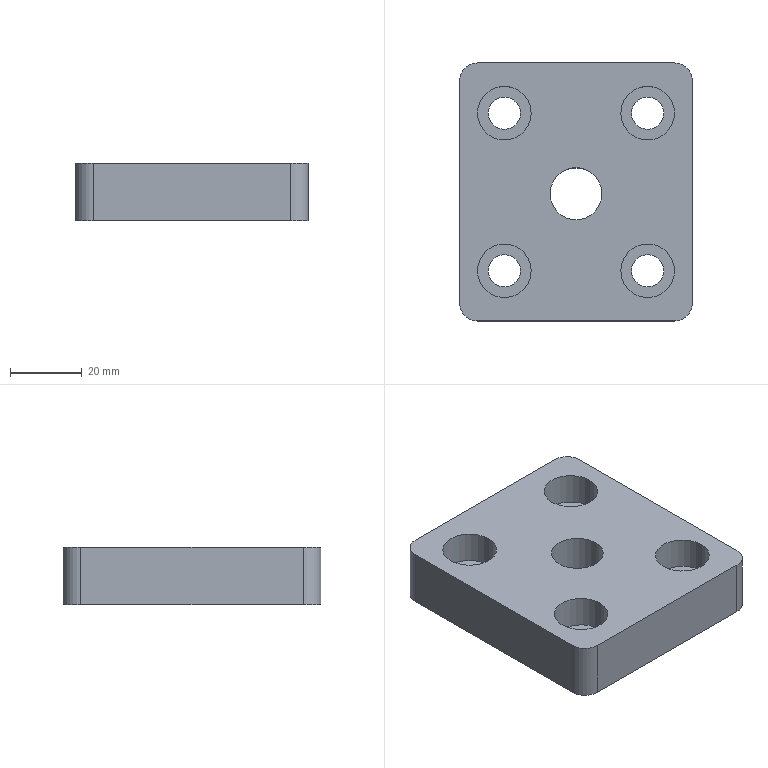Part | NX | features BREP 1 | 1 solid | 32 faces | box 65 x 72 x 16 mm | volume 63752 mm3 | cylinder 22 | plane 10 | commonest cylinder face diameters 9 x8 15 x8 10 x4 14.5 x2
STEP:
#1=CARTESIAN_POINT('',(7.25,-0.5,0.));
#2=VERTEX_POINT('',#1);
#3=CARTESIAN_POINT('',(-7.25,-0.5,0.));
#4=VERTEX_POINT('',#3);
#5=CARTESIAN_POINT('',(-0.000000218,-0.5,0.));
#6=DIRECTION('',(0.,0.,-1.));
#7=DIRECTION('',(-1.,0.,0.));
#8=AXIS2_PLACEMENT_3D('',#5,#6,#7);
#9=CIRCLE('',#8,7.25);
#10=EDGE_CURVE('',#2,#4,#9,.T.);
#11=ORIENTED_EDGE('',*,*,#10,.T.);
#12=CARTESIAN_POINT('',(-7.25,-0.5,16.));
#13=VERTEX_POINT('',#12);
#14=CARTESIAN_POINT('',(-7.25,-0.5,16.));
#15=DIRECTION('',(0.,0.,1.));
#16=VECTOR('',#15,1000.);
#17=LINE('',#14,#16);
#18=EDGE_CURVE('',#13,#4,#17,.F.);
#19=ORIENTED_EDGE('',*,*,#18,.F.);
#20=CARTESIAN_POINT('',(7.25,-0.5,16.));
#21=VERTEX_POINT('',#20);
#22=CARTESIAN_POINT('',(-0.000000218,-0.5,16.));
#23=DIRECTION('',(0.,0.,1.));
#24=DIRECTION('',(1.,0.,0.));
#25=AXIS2_PLACEMENT_3D('',#22,#23,#24);
#26=CIRCLE('',#25,7.25);
#27=EDGE_CURVE('',#13,#21,#26,.T.);
#28=ORIENTED_EDGE('',*,*,#27,.T.);
#29=CARTESIAN_POINT('',(7.25,-0.5,16.));
#30=DIRECTION('',(0.,0.,1.));
#31=VECTOR('',#30,1000.);
#32=LINE('',#29,#31);
#33=EDGE_CURVE('',#21,#2,#32,.F.);
#34=ORIENTED_EDGE('',*,*,#33,.T.);
#35=EDGE_LOOP('',(#11,#19,#28,#34));
#36=FACE_BOUND('',#35,.T.);
#37=CARTESIAN_POINT('',(-0.000000218,-0.5,16.));
#38=DIRECTION('',(0.,0.,1.));
#39=DIRECTION('',(1.,0.,0.));
#40=AXIS2_PLACEMENT_3D('',#37,#38,#39);
#41=CYLINDRICAL_SURFACE('',#40,7.25);
#42=ADVANCED_FACE('',(#36),#41,.F.);
#43=CARTESIAN_POINT('',(-27.5,22.,7.));
#44=VERTEX_POINT('',#43);
#45=CARTESIAN_POINT('',(-12.5,22.,7.));
#46=VERTEX_POINT('',#45);
#47=CARTESIAN_POINT('',(-20.,22.,7.));
#48=DIRECTION('',(0.,0.,1.));
#49=DIRECTION('',(1.,0.,0.));
#50=AXIS2_PLACEMENT_3D('',#47,#48,#49);
#51=CIRCLE('',#50,7.5);
#52=EDGE_CURVE('',#44,#46,#51,.T.);
#53=ORIENTED_EDGE('',*,*,#52,.F.);
#54=CARTESIAN_POINT('',(-27.5,22.,16.));
#55=VERTEX_POINT('',#54);
#56=CARTESIAN_POINT('',(-27.5,22.,16.));
#57=DIRECTION('',(0.,0.,1.));
#58=VECTOR('',#57,1000.);
#59=LINE('',#56,#58);
#60=EDGE_CURVE('',#55,#44,#59,.F.);
#61=ORIENTED_EDGE('',*,*,#60,.F.);
#62=CARTESIAN_POINT('',(-12.5,22.,16.));
#63=VERTEX_POINT('',#62);
#64=CARTESIAN_POINT('',(-20.,22.,16.));
#65=DIRECTION('',(0.,0.,1.));
#66=DIRECTION('',(1.,0.,0.));
#67=AXIS2_PLACEMENT_3D('',#64,#65,#66);
#68=CIRCLE('',#67,7.5);
#69=EDGE_CURVE('',#55,#63,#68,.T.);
#70=ORIENTED_EDGE('',*,*,#69,.T.);
#71=CARTESIAN_POINT('',(-12.5,22.,16.));
#72=DIRECTION('',(0.,0.,1.));
#73=VECTOR('',#72,1000.);
#74=LINE('',#71,#73);
#75=EDGE_CURVE('',#63,#46,#74,.F.);
#76=ORIENTED_EDGE('',*,*,#75,.T.);
#77=EDGE_LOOP('',(#53,#61,#70,#76));
#78=FACE_BOUND('',#77,.T.);
#79=CARTESIAN_POINT('',(-20.,22.,16.));
#80=DIRECTION('',(0.,0.,1.));
#81=DIRECTION('',(1.,0.,0.));
#82=AXIS2_PLACEMENT_3D('',#79,#80,#81);
#83=CYLINDRICAL_SURFACE('',#82,7.5);
#84=ADVANCED_FACE('',(#78),#83,.F.);
#85=CARTESIAN_POINT('',(-24.5,22.,0.));
#86=VERTEX_POINT('',#85);
#87=CARTESIAN_POINT('',(-15.5,22.,0.));
#88=VERTEX_POINT('',#87);
#89=CARTESIAN_POINT('',(-20.,22.,0.));
#90=DIRECTION('',(0.,0.,1.));
#91=DIRECTION('',(1.,0.,0.));
#92=AXIS2_PLACEMENT_3D('',#89,#90,#91);
#93=CIRCLE('',#92,4.5);
#94=EDGE_CURVE('',#86,#88,#93,.T.);
#95=ORIENTED_EDGE('',*,*,#94,.F.);
#96=CARTESIAN_POINT('',(-24.5,22.,7.));
#97=VERTEX_POINT('',#96);
#98=CARTESIAN_POINT('',(-24.5,22.,16.));
#99=DIRECTION('',(0.,0.,1.));
#100=VECTOR('',#99,1000.);
#101=LINE('',#98,#100);
#102=EDGE_CURVE('',#97,#86,#101,.F.);
#103=ORIENTED_EDGE('',*,*,#102,.F.);
#104=CARTESIAN_POINT('',(-15.5,22.,7.));
#105=VERTEX_POINT('',#104);
#106=CARTESIAN_POINT('',(-20.,22.,7.));
#107=DIRECTION('',(0.,0.,1.));
#108=DIRECTION('',(1.,0.,0.));
#109=AXIS2_PLACEMENT_3D('',#106,#107,#108);
#110=CIRCLE('',#109,4.5);
#111=EDGE_CURVE('',#97,#105,#110,.T.);
#112=ORIENTED_EDGE('',*,*,#111,.T.);
#113=CARTESIAN_POINT('',(-15.5,22.,16.));
#114=DIRECTION('',(0.,0.,1.));
#115=VECTOR('',#114,1000.);
#116=LINE('',#113,#115);
#117=EDGE_CURVE('',#105,#88,#116,.F.);
#118=ORIENTED_EDGE('',*,*,#117,.T.);
#119=EDGE_LOOP('',(#95,#103,#112,#118));
#120=FACE_BOUND('',#119,.T.);
#121=CARTESIAN_POINT('',(-20.,22.,16.));
#122=DIRECTION('',(0.,0.,1.));
#123=DIRECTION('',(1.,0.,0.));
#124=AXIS2_PLACEMENT_3D('',#121,#122,#123);
#125=CYLINDRICAL_SURFACE('',#124,4.5);
#126=ADVANCED_FACE('',(#120),#125,.F.);
#127=CARTESIAN_POINT('',(12.5,22.,7.));
#128=VERTEX_POINT('',#127);
#129=CARTESIAN_POINT('',(27.5,22.,7.));
#130=VERTEX_POINT('',#129);
#131=CARTESIAN_POINT('',(20.,22.,7.));
#132=DIRECTION('',(0.,0.,1.));
#133=DIRECTION('',(1.,0.,0.));
#134=AXIS2_PLACEMENT_3D('',#131,#132,#133);
#135=CIRCLE('',#134,7.5);
#136=EDGE_CURVE('',#128,#130,#135,.T.);
#137=ORIENTED_EDGE('',*,*,#136,.F.);
#138=CARTESIAN_POINT('',(12.5,22.,16.));
#139=VERTEX_POINT('',#138);
#140=CARTESIAN_POINT('',(12.5,22.,16.));
#141=DIRECTION('',(0.,0.,1.));
#142=VECTOR('',#141,1000.);
#143=LINE('',#140,#142);
#144=EDGE_CURVE('',#139,#128,#143,.F.);
#145=ORIENTED_EDGE('',*,*,#144,.F.);
#146=CARTESIAN_POINT('',(27.5,22.,16.));
#147=VERTEX_POINT('',#146);
#148=CARTESIAN_POINT('',(20.,22.,16.));
#149=DIRECTION('',(0.,0.,1.));
#150=DIRECTION('',(1.,0.,0.));
#151=AXIS2_PLACEMENT_3D('',#148,#149,#150);
#152=CIRCLE('',#151,7.5);
#153=EDGE_CURVE('',#139,#147,#152,.T.);
#154=ORIENTED_EDGE('',*,*,#153,.T.);
#155=CARTESIAN_POINT('',(27.5,22.,16.));
#156=DIRECTION('',(0.,0.,1.));
#157=VECTOR('',#156,1000.);
#158=LINE('',#155,#157);
#159=EDGE_CURVE('',#147,#130,#158,.F.);
#160=ORIENTED_EDGE('',*,*,#159,.T.);
#161=EDGE_LOOP('',(#137,#145,#154,#160));
#162=FACE_BOUND('',#161,.T.);
#163=CARTESIAN_POINT('',(20.,22.,16.));
#164=DIRECTION('',(0.,0.,1.));
#165=DIRECTION('',(1.,0.,0.));
#166=AXIS2_PLACEMENT_3D('',#163,#164,#165);
#167=CYLINDRICAL_SURFACE('',#166,7.5);
#168=ADVANCED_FACE('',(#162),#167,.F.);
#169=CARTESIAN_POINT('',(15.5,22.,0.));
#170=VERTEX_POINT('',#169);
#171=CARTESIAN_POINT('',(24.5,22.,0.));
#172=VERTEX_POINT('',#171);
#173=CARTESIAN_POINT('',(20.,22.,0.));
#174=DIRECTION('',(0.,0.,1.));
#175=DIRECTION('',(1.,0.,0.));
#176=AXIS2_PLACEMENT_3D('',#173,#174,#175);
#177=CIRCLE('',#176,4.5);
#178=EDGE_CURVE('',#170,#172,#177,.T.);
#179=ORIENTED_EDGE('',*,*,#178,.F.);
#180=CARTESIAN_POINT('',(15.5,22.,7.));
#181=VERTEX_POINT('',#180);
#182=CARTESIAN_POINT('',(15.5,22.,16.));
#183=DIRECTION('',(0.,0.,1.));
#184=VECTOR('',#183,1000.);
#185=LINE('',#182,#184);
#186=EDGE_CURVE('',#181,#170,#185,.F.);
#187=ORIENTED_EDGE('',*,*,#186,.F.);
#188=CARTESIAN_POINT('',(24.5,22.,7.));
#189=VERTEX_POINT('',#188);
#190=CARTESIAN_POINT('',(20.,22.,7.));
#191=DIRECTION('',(0.,0.,1.));
#192=DIRECTION('',(1.,0.,0.));
#193=AXIS2_PLACEMENT_3D('',#190,#191,#192);
#194=CIRCLE('',#193,4.5);
#195=EDGE_CURVE('',#181,#189,#194,.T.);
#196=ORIENTED_EDGE('',*,*,#195,.T.);
#197=CARTESIAN_POINT('',(24.5,22.,16.));
#198=DIRECTION('',(0.,0.,1.));
#199=VECTOR('',#198,1000.);
#200=LINE('',#197,#199);
#201=EDGE_CURVE('',#189,#172,#200,.F.);
#202=ORIENTED_EDGE('',*,*,#201,.T.);
#203=EDGE_LOOP('',(#179,#187,#196,#202));
#204=FACE_BOUND('',#203,.T.);
#205=CARTESIAN_POINT('',(20.,22.,16.));
#206=DIRECTION('',(0.,0.,1.));
#207=DIRECTION('',(1.,0.,0.));
#208=AXIS2_PLACEMENT_3D('',#205,#206,#207);
#209=CYLINDRICAL_SURFACE('',#208,4.5);
#210=ADVANCED_FACE('',(#204),#209,.F.);
#211=CARTESIAN_POINT('',(-27.5,-22.,7.));
#212=VERTEX_POINT('',#211);
#213=CARTESIAN_POINT('',(-12.5,-22.,7.));
#214=VERTEX_POINT('',#213);
#215=CARTESIAN_POINT('',(-20.,-22.,7.));
#216=DIRECTION('',(0.,0.,1.));
#217=DIRECTION('',(1.,0.,0.));
#218=AXIS2_PLACEMENT_3D('',#215,#216,#217);
#219=CIRCLE('',#218,7.5);
#220=EDGE_CURVE('',#212,#214,#219,.T.);
#221=ORIENTED_EDGE('',*,*,#220,.F.);
#222=CARTESIAN_POINT('',(-27.5,-22.,16.));
#223=VERTEX_POINT('',#222);
#224=CARTESIAN_POINT('',(-27.5,-22.,16.));
#225=DIRECTION('',(0.,0.,1.));
#226=VECTOR('',#225,1000.);
#227=LINE('',#224,#226);
#228=EDGE_CURVE('',#223,#212,#227,.F.);
#229=ORIENTED_EDGE('',*,*,#228,.F.);
#230=CARTESIAN_POINT('',(-12.5,-22.,16.));
#231=VERTEX_POINT('',#230);
#232=CARTESIAN_POINT('',(-20.,-22.,16.));
#233=DIRECTION('',(0.,0.,1.));
#234=DIRECTION('',(1.,0.,0.));
#235=AXIS2_PLACEMENT_3D('',#232,#233,#234);
#236=CIRCLE('',#235,7.5);
#237=EDGE_CURVE('',#223,#231,#236,.T.);
#238=ORIENTED_EDGE('',*,*,#237,.T.);
#239=CARTESIAN_POINT('',(-12.5,-22.,16.));
#240=DIRECTION('',(0.,0.,1.));
#241=VECTOR('',#240,1000.);
#242=LINE('',#239,#241);
#243=EDGE_CURVE('',#231,#214,#242,.F.);
#244=ORIENTED_EDGE('',*,*,#243,.T.);
#245=EDGE_LOOP('',(#221,#229,#238,#244));
#246=FACE_BOUND('',#245,.T.);
#247=CARTESIAN_POINT('',(-20.,-22.,16.));
#248=DIRECTION('',(0.,0.,1.));
#249=DIRECTION('',(1.,0.,0.));
#250=AXIS2_PLACEMENT_3D('',#247,#248,#249);
#251=CYLINDRICAL_SURFACE('',#250,7.5);
#252=ADVANCED_FACE('',(#246),#251,.F.);
#253=CARTESIAN_POINT('',(-24.5,-22.,0.));
#254=VERTEX_POINT('',#253);
#255=CARTESIAN_POINT('',(-15.5,-22.,0.));
#256=VERTEX_POINT('',#255);
#257=CARTESIAN_POINT('',(-20.,-22.,0.));
#258=DIRECTION('',(0.,0.,1.));
#259=DIRECTION('',(1.,0.,0.));
#260=AXIS2_PLACEMENT_3D('',#257,#258,#259);
#261=CIRCLE('',#260,4.5);
#262=EDGE_CURVE('',#254,#256,#261,.T.);
#263=ORIENTED_EDGE('',*,*,#262,.F.);
#264=CARTESIAN_POINT('',(-24.5,-22.,7.));
#265=VERTEX_POINT('',#264);
#266=CARTESIAN_POINT('',(-24.5,-22.,16.));
#267=DIRECTION('',(0.,0.,1.));
#268=VECTOR('',#267,1000.);
#269=LINE('',#266,#268);
#270=EDGE_CURVE('',#265,#254,#269,.F.);
#271=ORIENTED_EDGE('',*,*,#270,.F.);
#272=CARTESIAN_POINT('',(-15.5,-22.,7.));
#273=VERTEX_POINT('',#272);
#274=CARTESIAN_POINT('',(-20.,-22.,7.));
#275=DIRECTION('',(0.,0.,1.));
#276=DIRECTION('',(1.,0.,0.));
#277=AXIS2_PLACEMENT_3D('',#274,#275,#276);
#278=CIRCLE('',#277,4.5);
#279=EDGE_CURVE('',#265,#273,#278,.T.);
#280=ORIENTED_EDGE('',*,*,#279,.T.);
#281=CARTESIAN_POINT('',(-15.5,-22.,16.));
#282=DIRECTION('',(0.,0.,1.));
#283=VECTOR('',#282,1000.);
#284=LINE('',#281,#283);
#285=EDGE_CURVE('',#273,#256,#284,.F.);
#286=ORIENTED_EDGE('',*,*,#285,.T.);
#287=EDGE_LOOP('',(#263,#271,#280,#286));
#288=FACE_BOUND('',#287,.T.);
#289=CARTESIAN_POINT('',(-20.,-22.,16.));
#290=DIRECTION('',(0.,0.,1.));
#291=DIRECTION('',(1.,0.,0.));
#292=AXIS2_PLACEMENT_3D('',#289,#290,#291);
#293=CYLINDRICAL_SURFACE('',#292,4.5);
#294=ADVANCED_FACE('',(#288),#293,.F.);
#295=CARTESIAN_POINT('',(12.5,-22.,7.));
#296=VERTEX_POINT('',#295);
#297=CARTESIAN_POINT('',(27.5,-22.,7.));
#298=VERTEX_POINT('',#297);
#299=CARTESIAN_POINT('',(20.,-22.,7.));
#300=DIRECTION('',(0.,0.,1.));
#301=DIRECTION('',(1.,0.,0.));
#302=AXIS2_PLACEMENT_3D('',#299,#300,#301);
#303=CIRCLE('',#302,7.5);
#304=EDGE_CURVE('',#296,#298,#303,.T.);
#305=ORIENTED_EDGE('',*,*,#304,.F.);
#306=CARTESIAN_POINT('',(12.5,-22.,16.));
#307=VERTEX_POINT('',#306);
#308=CARTESIAN_POINT('',(12.5,-22.,16.));
#309=DIRECTION('',(0.,0.,1.));
#310=VECTOR('',#309,1000.);
#311=LINE('',#308,#310);
#312=EDGE_CURVE('',#307,#296,#311,.F.);
#313=ORIENTED_EDGE('',*,*,#312,.F.);
#314=CARTESIAN_POINT('',(27.5,-22.,16.));
#315=VERTEX_POINT('',#314);
#316=CARTESIAN_POINT('',(20.,-22.,16.));
#317=DIRECTION('',(0.,0.,1.));
#318=DIRECTION('',(1.,0.,0.));
#319=AXIS2_PLACEMENT_3D('',#316,#317,#318);
#320=CIRCLE('',#319,7.5);
#321=EDGE_CURVE('',#307,#315,#320,.T.);
#322=ORIENTED_EDGE('',*,*,#321,.T.);
#323=CARTESIAN_POINT('',(27.5,-22.,16.));
#324=DIRECTION('',(0.,0.,1.));
#325=VECTOR('',#324,1000.);
#326=LINE('',#323,#325);
#327=EDGE_CURVE('',#315,#298,#326,.F.);
#328=ORIENTED_EDGE('',*,*,#327,.T.);
#329=EDGE_LOOP('',(#305,#313,#322,#328));
#330=FACE_BOUND('',#329,.T.);
#331=CARTESIAN_POINT('',(20.,-22.,16.));
#332=DIRECTION('',(0.,0.,1.));
#333=DIRECTION('',(1.,0.,0.));
#334=AXIS2_PLACEMENT_3D('',#331,#332,#333);
#335=CYLINDRICAL_SURFACE('',#334,7.5);
#336=ADVANCED_FACE('',(#330),#335,.F.);
#337=CARTESIAN_POINT('',(15.5,-22.,0.));
#338=VERTEX_POINT('',#337);
#339=CARTESIAN_POINT('',(24.5,-22.,0.));
#340=VERTEX_POINT('',#339);
#341=CARTESIAN_POINT('',(20.,-22.,0.));
#342=DIRECTION('',(0.,0.,1.));
#343=DIRECTION('',(1.,0.,0.));
#344=AXIS2_PLACEMENT_3D('',#341,#342,#343);
#345=CIRCLE('',#344,4.5);
#346=EDGE_CURVE('',#338,#340,#345,.T.);
#347=ORIENTED_EDGE('',*,*,#346,.F.);
#348=CARTESIAN_POINT('',(15.5,-22.,7.));
#349=VERTEX_POINT('',#348);
#350=CARTESIAN_POINT('',(15.5,-22.,16.));
#351=DIRECTION('',(0.,0.,1.));
#352=VECTOR('',#351,1000.);
#353=LINE('',#350,#352);
#354=EDGE_CURVE('',#349,#338,#353,.F.);
#355=ORIENTED_EDGE('',*,*,#354,.F.);
#356=CARTESIAN_POINT('',(24.5,-22.,7.));
#357=VERTEX_POINT('',#356);
#358=CARTESIAN_POINT('',(20.,-22.,7.));
#359=DIRECTION('',(0.,0.,1.));
#360=DIRECTION('',(1.,0.,0.));
#361=AXIS2_PLACEMENT_3D('',#358,#359,#360);
#362=CIRCLE('',#361,4.5);
#363=EDGE_CURVE('',#349,#357,#362,.T.);
#364=ORIENTED_EDGE('',*,*,#363,.T.);
#365=CARTESIAN_POINT('',(24.5,-22.,16.));
#366=DIRECTION('',(0.,0.,1.));
#367=VECTOR('',#366,1000.);
#368=LINE('',#365,#367);
#369=EDGE_CURVE('',#357,#340,#368,.F.);
#370=ORIENTED_EDGE('',*,*,#369,.T.);
#371=EDGE_LOOP('',(#347,#355,#364,#370));
#372=FACE_BOUND('',#371,.T.);
#373=CARTESIAN_POINT('',(20.,-22.,16.));
#374=DIRECTION('',(0.,0.,1.));
#375=DIRECTION('',(1.,0.,0.));
#376=AXIS2_PLACEMENT_3D('',#373,#374,#375);
#377=CYLINDRICAL_SURFACE('',#376,4.5);
#378=ADVANCED_FACE('',(#372),#377,.F.);
#379=CARTESIAN_POINT('',(32.5,-31.,0.));
#380=VERTEX_POINT('',#379);
#381=CARTESIAN_POINT('',(32.5,31.,0.));
#382=VERTEX_POINT('',#381);
#383=CARTESIAN_POINT('',(32.5,-36.,0.));
#384=DIRECTION('',(0.,1.,0.));
#385=VECTOR('',#384,1000.);
#386=LINE('',#383,#385);
#387=EDGE_CURVE('',#380,#382,#386,.T.);
#388=ORIENTED_EDGE('',*,*,#387,.T.);
#389=CARTESIAN_POINT('',(32.5,31.,16.));
#390=VERTEX_POINT('',#389);
#391=CARTESIAN_POINT('',(32.5,31.,16.));
#392=DIRECTION('',(0.,0.,1.));
#393=VECTOR('',#392,1000.);
#394=LINE('',#391,#393);
#395=EDGE_CURVE('',#382,#390,#394,.T.);
#396=ORIENTED_EDGE('',*,*,#395,.T.);
#397=CARTESIAN_POINT('',(32.5,-31.,16.));
#398=VERTEX_POINT('',#397);
#399=CARTESIAN_POINT('',(32.5,-36.,16.));
#400=DIRECTION('',(0.,1.,0.));
#401=VECTOR('',#400,1000.);
#402=LINE('',#399,#401);
#403=EDGE_CURVE('',#398,#390,#402,.T.);
#404=ORIENTED_EDGE('',*,*,#403,.F.);
#405=CARTESIAN_POINT('',(32.5,-31.,16.));
#406=DIRECTION('',(0.,0.,-1.));
#407=VECTOR('',#406,1000.);
#408=LINE('',#405,#407);
#409=EDGE_CURVE('',#398,#380,#408,.T.);
#410=ORIENTED_EDGE('',*,*,#409,.T.);
#411=EDGE_LOOP('',(#388,#396,#404,#410));
#412=FACE_BOUND('',#411,.T.);
#413=CARTESIAN_POINT('',(32.5,-36.,16.));
#414=DIRECTION('',(-1.,0.,0.));
#415=DIRECTION('',(0.,0.,1.));
#416=AXIS2_PLACEMENT_3D('',#413,#414,#415);
#417=PLANE('',#416);
#418=ADVANCED_FACE('',(#412),#417,.F.);
#419=CARTESIAN_POINT('',(27.5,36.,16.));
#420=VERTEX_POINT('',#419);
#421=CARTESIAN_POINT('',(-27.5,36.,16.));
#422=VERTEX_POINT('',#421);
#423=CARTESIAN_POINT('',(-32.5,36.,16.));
#424=DIRECTION('',(-1.,0.,0.));
#425=VECTOR('',#424,1000.);
#426=LINE('',#423,#425);
#427=EDGE_CURVE('',#420,#422,#426,.T.);
#428=ORIENTED_EDGE('',*,*,#427,.F.);
#429=CARTESIAN_POINT('',(27.5,36.,0.));
#430=VERTEX_POINT('',#429);
#431=CARTESIAN_POINT('',(27.5,36.,16.));
#432=DIRECTION('',(0.,0.,-1.));
#433=VECTOR('',#432,1000.);
#434=LINE('',#431,#433);
#435=EDGE_CURVE('',#420,#430,#434,.T.);
#436=ORIENTED_EDGE('',*,*,#435,.T.);
#437=CARTESIAN_POINT('',(-27.5,36.,0.));
#438=VERTEX_POINT('',#437);
#439=CARTESIAN_POINT('',(-32.5,36.,0.));
#440=DIRECTION('',(-1.,0.,0.));
#441=VECTOR('',#440,1000.);
#442=LINE('',#439,#441);
#443=EDGE_CURVE('',#430,#438,#442,.T.);
#444=ORIENTED_EDGE('',*,*,#443,.T.);
#445=CARTESIAN_POINT('',(-27.5,36.,16.));
#446=DIRECTION('',(0.,0.,1.));
#447=VECTOR('',#446,1000.);
#448=LINE('',#445,#447);
#449=EDGE_CURVE('',#438,#422,#448,.T.);
#450=ORIENTED_EDGE('',*,*,#449,.T.);
#451=EDGE_LOOP('',(#428,#436,#444,#450));
#452=FACE_BOUND('',#451,.T.);
#453=CARTESIAN_POINT('',(-32.5,36.,16.));
#454=DIRECTION('',(0.,-1.,0.));
#455=DIRECTION('',(0.,0.,-1.));
#456=AXIS2_PLACEMENT_3D('',#453,#454,#455);
#457=PLANE('',#456);
#458=ADVANCED_FACE('',(#452),#457,.F.);
#459=CARTESIAN_POINT('',(-32.5,31.,0.));
#460=VERTEX_POINT('',#459);
#461=CARTESIAN_POINT('',(-32.5,-31.,0.));
#462=VERTEX_POINT('',#461);
#463=CARTESIAN_POINT('',(-32.5,-36.,0.));
#464=DIRECTION('',(0.,-1.,0.));
#465=VECTOR('',#464,1000.);
#466=LINE('',#463,#465);
#467=EDGE_CURVE('',#460,#462,#466,.T.);
#468=ORIENTED_EDGE('',*,*,#467,.T.);
#469=CARTESIAN_POINT('',(-32.5,-31.,16.));
#470=VERTEX_POINT('',#469);
#471=CARTESIAN_POINT('',(-32.5,-31.,16.));
#472=DIRECTION('',(0.,0.,1.));
#473=VECTOR('',#472,1000.);
#474=LINE('',#471,#473);
#475=EDGE_CURVE('',#462,#470,#474,.T.);
#476=ORIENTED_EDGE('',*,*,#475,.T.);
#477=CARTESIAN_POINT('',(-32.5,31.,16.));
#478=VERTEX_POINT('',#477);
#479=CARTESIAN_POINT('',(-32.5,-36.,16.));
#480=DIRECTION('',(0.,-1.,0.));
#481=VECTOR('',#480,1000.);
#482=LINE('',#479,#481);
#483=EDGE_CURVE('',#478,#470,#482,.T.);
#484=ORIENTED_EDGE('',*,*,#483,.F.);
#485=CARTESIAN_POINT('',(-32.5,31.,16.));
#486=DIRECTION('',(0.,0.,-1.));
#487=VECTOR('',#486,1000.);
#488=LINE('',#485,#487);
#489=EDGE_CURVE('',#478,#460,#488,.T.);
#490=ORIENTED_EDGE('',*,*,#489,.T.);
#491=EDGE_LOOP('',(#468,#476,#484,#490));
#492=FACE_BOUND('',#491,.T.);
#493=CARTESIAN_POINT('',(-32.5,-36.,16.));
#494=DIRECTION('',(1.,0.,0.));
#495=DIRECTION('',(0.,1.,0.));
#496=AXIS2_PLACEMENT_3D('',#493,#494,#495);
#497=PLANE('',#496);
#498=ADVANCED_FACE('',(#492),#497,.F.);
#499=CARTESIAN_POINT('',(-27.5,-36.,0.));
#500=VERTEX_POINT('',#499);
#501=CARTESIAN_POINT('',(27.5,-36.,0.));
#502=VERTEX_POINT('',#501);
#503=CARTESIAN_POINT('',(-32.5,-36.,0.));
#504=DIRECTION('',(1.,0.,0.));
#505=VECTOR('',#504,1000.);
#506=LINE('',#503,#505);
#507=EDGE_CURVE('',#500,#502,#506,.T.);
#508=ORIENTED_EDGE('',*,*,#507,.T.);
#509=CARTESIAN_POINT('',(27.5,-36.,16.));
#510=VERTEX_POINT('',#509);
#511=CARTESIAN_POINT('',(27.5,-36.,16.));
#512=DIRECTION('',(0.,0.,1.));
#513=VECTOR('',#512,1000.);
#514=LINE('',#511,#513);
#515=EDGE_CURVE('',#502,#510,#514,.T.);
#516=ORIENTED_EDGE('',*,*,#515,.T.);
#517=CARTESIAN_POINT('',(-27.5,-36.,16.));
#518=VERTEX_POINT('',#517);
#519=CARTESIAN_POINT('',(-32.5,-36.,16.));
#520=DIRECTION('',(1.,0.,0.));
#521=VECTOR('',#520,1000.);
#522=LINE('',#519,#521);
#523=EDGE_CURVE('',#518,#510,#522,.T.);
#524=ORIENTED_EDGE('',*,*,#523,.F.);
#525=CARTESIAN_POINT('',(-27.5,-36.,16.));
#526=DIRECTION('',(0.,0.,-1.));
#527=VECTOR('',#526,1000.);
#528=LINE('',#525,#527);
#529=EDGE_CURVE('',#518,#500,#528,.T.);
#530=ORIENTED_EDGE('',*,*,#529,.T.);
#531=EDGE_LOOP('',(#508,#516,#524,#530));
#532=FACE_BOUND('',#531,.T.);
#533=CARTESIAN_POINT('',(-32.5,-36.,16.));
#534=DIRECTION('',(0.,1.,0.));
#535=DIRECTION('',(1.,0.,0.));
#536=AXIS2_PLACEMENT_3D('',#533,#534,#535);
#537=PLANE('',#536);
#538=ADVANCED_FACE('',(#532),#537,.F.);
#539=ORIENTED_EDGE('',*,*,#403,.T.);
#540=CARTESIAN_POINT('',(27.5,31.,16.));
#541=DIRECTION('',(0.,0.,1.));
#542=DIRECTION('',(-1.,0.,0.));
#543=AXIS2_PLACEMENT_3D('',#540,#541,#542);
#544=CIRCLE('',#543,5.);
#545=EDGE_CURVE('',#390,#420,#544,.T.);
#546=ORIENTED_EDGE('',*,*,#545,.T.);
#547=ORIENTED_EDGE('',*,*,#427,.T.);
#548=CARTESIAN_POINT('',(-27.5,31.,16.));
#549=DIRECTION('',(0.,0.,1.));
#550=DIRECTION('',(-1.,0.,0.));
#551=AXIS2_PLACEMENT_3D('',#548,#549,#550);
#552=CIRCLE('',#551,5.);
#553=EDGE_CURVE('',#422,#478,#552,.T.);
#554=ORIENTED_EDGE('',*,*,#553,.T.);
#555=ORIENTED_EDGE('',*,*,#483,.T.);
#556=CARTESIAN_POINT('',(-27.5,-31.,16.));
#557=DIRECTION('',(0.,0.,1.));
#558=DIRECTION('',(-1.,0.,0.));
#559=AXIS2_PLACEMENT_3D('',#556,#557,#558);
#560=CIRCLE('',#559,5.);
#561=EDGE_CURVE('',#470,#518,#560,.T.);
#562=ORIENTED_EDGE('',*,*,#561,.T.);
#563=ORIENTED_EDGE('',*,*,#523,.T.);
#564=CARTESIAN_POINT('',(27.5,-31.,16.));
#565=DIRECTION('',(0.,0.,1.));
#566=DIRECTION('',(-1.,0.,0.));
#567=AXIS2_PLACEMENT_3D('',#564,#565,#566);
#568=CIRCLE('',#567,5.);
#569=EDGE_CURVE('',#510,#398,#568,.T.);
#570=ORIENTED_EDGE('',*,*,#569,.T.);
#571=EDGE_LOOP('',(#539,#546,#547,#554,#555,#562,#563,#570));
#572=FACE_BOUND('',#571,.T.);
#573=CARTESIAN_POINT('',(-0.000000218,-0.5,16.));
#574=DIRECTION('',(0.,0.,1.));
#575=DIRECTION('',(1.,0.,0.));
#576=AXIS2_PLACEMENT_3D('',#573,#574,#575);
#577=CIRCLE('',#576,7.25);
#578=EDGE_CURVE('',#21,#13,#577,.T.);
#579=ORIENTED_EDGE('',*,*,#578,.F.);
#580=ORIENTED_EDGE('',*,*,#27,.F.);
#581=EDGE_LOOP('',(#579,#580));
#582=FACE_BOUND('',#581,.T.);
#583=CARTESIAN_POINT('',(-20.,22.,16.));
#584=DIRECTION('',(0.,0.,1.));
#585=DIRECTION('',(1.,0.,0.));
#586=AXIS2_PLACEMENT_3D('',#583,#584,#585);
#587=CIRCLE('',#586,7.5);
#588=EDGE_CURVE('',#63,#55,#587,.T.);
#589=ORIENTED_EDGE('',*,*,#588,.F.);
#590=ORIENTED_EDGE('',*,*,#69,.F.);
#591=EDGE_LOOP('',(#589,#590));
#592=FACE_BOUND('',#591,.T.);
#593=CARTESIAN_POINT('',(20.,22.,16.));
#594=DIRECTION('',(0.,0.,1.));
#595=DIRECTION('',(1.,0.,0.));
#596=AXIS2_PLACEMENT_3D('',#593,#594,#595);
#597=CIRCLE('',#596,7.5);
#598=EDGE_CURVE('',#147,#139,#597,.T.);
#599=ORIENTED_EDGE('',*,*,#598,.F.);
#600=ORIENTED_EDGE('',*,*,#153,.F.);
#601=EDGE_LOOP('',(#599,#600));
#602=FACE_BOUND('',#601,.T.);
#603=CARTESIAN_POINT('',(-20.,-22.,16.));
#604=DIRECTION('',(0.,0.,1.));
#605=DIRECTION('',(1.,0.,0.));
#606=AXIS2_PLACEMENT_3D('',#603,#604,#605);
#607=CIRCLE('',#606,7.5);
#608=EDGE_CURVE('',#231,#223,#607,.T.);
#609=ORIENTED_EDGE('',*,*,#608,.F.);
#610=ORIENTED_EDGE('',*,*,#237,.F.);
#611=EDGE_LOOP('',(#609,#610));
#612=FACE_BOUND('',#611,.T.);
#613=CARTESIAN_POINT('',(20.,-22.,16.));
#614=DIRECTION('',(0.,0.,1.));
#615=DIRECTION('',(1.,0.,0.));
#616=AXIS2_PLACEMENT_3D('',#613,#614,#615);
#617=CIRCLE('',#616,7.5);
#618=EDGE_CURVE('',#315,#307,#617,.T.);
#619=ORIENTED_EDGE('',*,*,#618,.F.);
#620=ORIENTED_EDGE('',*,*,#321,.F.);
#621=EDGE_LOOP('',(#619,#620));
#622=FACE_BOUND('',#621,.T.);
#623=CARTESIAN_POINT('',(0.,0.,16.));
#624=DIRECTION('',(0.,0.,-1.));
#625=DIRECTION('',(0.,-1.,0.));
#626=AXIS2_PLACEMENT_3D('',#623,#624,#625);
#627=PLANE('',#626);
#628=ADVANCED_FACE('',(#572,#582,#592,#602,#612,#622),#627,.F.);
#629=ORIENTED_EDGE('',*,*,#443,.F.);
#630=CARTESIAN_POINT('',(27.5,31.,0.));
#631=DIRECTION('',(0.,0.,-1.));
#632=DIRECTION('',(-1.,0.,0.));
#633=AXIS2_PLACEMENT_3D('',#630,#631,#632);
#634=CIRCLE('',#633,5.);
#635=EDGE_CURVE('',#430,#382,#634,.T.);
#636=ORIENTED_EDGE('',*,*,#635,.T.);
#637=ORIENTED_EDGE('',*,*,#387,.F.);
#638=CARTESIAN_POINT('',(27.5,-31.,0.));
#639=DIRECTION('',(0.,0.,-1.));
#640=DIRECTION('',(-1.,0.,0.));
#641=AXIS2_PLACEMENT_3D('',#638,#639,#640);
#642=CIRCLE('',#641,5.);
#643=EDGE_CURVE('',#380,#502,#642,.T.);
#644=ORIENTED_EDGE('',*,*,#643,.T.);
#645=ORIENTED_EDGE('',*,*,#507,.F.);
#646=CARTESIAN_POINT('',(-27.5,-31.,0.));
#647=DIRECTION('',(0.,0.,-1.));
#648=DIRECTION('',(-1.,0.,0.));
#649=AXIS2_PLACEMENT_3D('',#646,#647,#648);
#650=CIRCLE('',#649,5.);
#651=EDGE_CURVE('',#500,#462,#650,.T.);
#652=ORIENTED_EDGE('',*,*,#651,.T.);
#653=ORIENTED_EDGE('',*,*,#467,.F.);
#654=CARTESIAN_POINT('',(-27.5,31.,0.));
#655=DIRECTION('',(0.,0.,-1.));
#656=DIRECTION('',(-1.,0.,0.));
#657=AXIS2_PLACEMENT_3D('',#654,#655,#656);
#658=CIRCLE('',#657,5.);
#659=EDGE_CURVE('',#460,#438,#658,.T.);
#660=ORIENTED_EDGE('',*,*,#659,.T.);
#661=EDGE_LOOP('',(#629,#636,#637,#644,#645,#652,#653,#660));
#662=FACE_BOUND('',#661,.T.);
#663=ORIENTED_EDGE('',*,*,#10,.F.);
#664=CARTESIAN_POINT('',(-0.000000218,-0.5,0.));
#665=DIRECTION('',(0.,0.,-1.));
#666=DIRECTION('',(-1.,0.,0.));
#667=AXIS2_PLACEMENT_3D('',#664,#665,#666);
#668=CIRCLE('',#667,7.25);
#669=EDGE_CURVE('',#4,#2,#668,.T.);
#670=ORIENTED_EDGE('',*,*,#669,.F.);
#671=EDGE_LOOP('',(#663,#670));
#672=FACE_BOUND('',#671,.T.);
#673=CARTESIAN_POINT('',(-20.,22.,0.));
#674=DIRECTION('',(0.,0.,1.));
#675=DIRECTION('',(1.,0.,0.));
#676=AXIS2_PLACEMENT_3D('',#673,#674,#675);
#677=CIRCLE('',#676,4.5);
#678=EDGE_CURVE('',#88,#86,#677,.T.);
#679=ORIENTED_EDGE('',*,*,#678,.T.);
#680=ORIENTED_EDGE('',*,*,#94,.T.);
#681=EDGE_LOOP('',(#679,#680));
#682=FACE_BOUND('',#681,.T.);
#683=CARTESIAN_POINT('',(20.,22.,0.));
#684=DIRECTION('',(0.,0.,1.));
#685=DIRECTION('',(1.,0.,0.));
#686=AXIS2_PLACEMENT_3D('',#683,#684,#685);
#687=CIRCLE('',#686,4.5);
#688=EDGE_CURVE('',#172,#170,#687,.T.);
#689=ORIENTED_EDGE('',*,*,#688,.T.);
#690=ORIENTED_EDGE('',*,*,#178,.T.);
#691=EDGE_LOOP('',(#689,#690));
#692=FACE_BOUND('',#691,.T.);
#693=CARTESIAN_POINT('',(-20.,-22.,0.));
#694=DIRECTION('',(0.,0.,1.));
#695=DIRECTION('',(1.,0.,0.));
#696=AXIS2_PLACEMENT_3D('',#693,#694,#695);
#697=CIRCLE('',#696,4.5);
#698=EDGE_CURVE('',#256,#254,#697,.T.);
#699=ORIENTED_EDGE('',*,*,#698,.T.);
#700=ORIENTED_EDGE('',*,*,#262,.T.);
#701=EDGE_LOOP('',(#699,#700));
#702=FACE_BOUND('',#701,.T.);
#703=CARTESIAN_POINT('',(20.,-22.,0.));
#704=DIRECTION('',(0.,0.,1.));
#705=DIRECTION('',(1.,0.,0.));
#706=AXIS2_PLACEMENT_3D('',#703,#704,#705);
#707=CIRCLE('',#706,4.5);
#708=EDGE_CURVE('',#340,#338,#707,.T.);
#709=ORIENTED_EDGE('',*,*,#708,.T.);
#710=ORIENTED_EDGE('',*,*,#346,.T.);
#711=EDGE_LOOP('',(#709,#710));
#712=FACE_BOUND('',#711,.T.);
#713=CARTESIAN_POINT('',(0.,0.,0.));
#714=DIRECTION('',(0.,0.,-1.));
#715=DIRECTION('',(0.,-1.,0.));
#716=AXIS2_PLACEMENT_3D('',#713,#714,#715);
#717=PLANE('',#716);
#718=ADVANCED_FACE('',(#662,#672,#682,#692,#702,#712),#717,.T.);
#719=ORIENTED_EDGE('',*,*,#354,.T.);
#720=ORIENTED_EDGE('',*,*,#708,.F.);
#721=ORIENTED_EDGE('',*,*,#369,.F.);
#722=CARTESIAN_POINT('',(20.,-22.,7.));
#723=DIRECTION('',(0.,0.,1.));
#724=DIRECTION('',(1.,0.,0.));
#725=AXIS2_PLACEMENT_3D('',#722,#723,#724);
#726=CIRCLE('',#725,4.5);
#727=EDGE_CURVE('',#357,#349,#726,.T.);
#728=ORIENTED_EDGE('',*,*,#727,.T.);
#729=EDGE_LOOP('',(#719,#720,#721,#728));
#730=FACE_BOUND('',#729,.T.);
#731=CARTESIAN_POINT('',(20.,-22.,16.));
#732=DIRECTION('',(0.,0.,1.));
#733=DIRECTION('',(1.,0.,0.));
#734=AXIS2_PLACEMENT_3D('',#731,#732,#733);
#735=CYLINDRICAL_SURFACE('',#734,4.5);
#736=ADVANCED_FACE('',(#730),#735,.F.);
#737=CARTESIAN_POINT('',(20.,-22.,7.));
#738=DIRECTION('',(0.,0.,1.));
#739=DIRECTION('',(1.,0.,0.));
#740=AXIS2_PLACEMENT_3D('',#737,#738,#739);
#741=CIRCLE('',#740,7.5);
#742=EDGE_CURVE('',#298,#296,#741,.T.);
#743=ORIENTED_EDGE('',*,*,#742,.T.);
#744=ORIENTED_EDGE('',*,*,#304,.T.);
#745=EDGE_LOOP('',(#743,#744));
#746=FACE_BOUND('',#745,.T.);
#747=ORIENTED_EDGE('',*,*,#727,.F.);
#748=ORIENTED_EDGE('',*,*,#363,.F.);
#749=EDGE_LOOP('',(#747,#748));
#750=FACE_BOUND('',#749,.T.);
#751=CARTESIAN_POINT('',(24.5,-22.,7.));
#752=DIRECTION('',(0.,0.,-1.));
#753=DIRECTION('',(0.,-1.,0.));
#754=AXIS2_PLACEMENT_3D('',#751,#752,#753);
#755=PLANE('',#754);
#756=ADVANCED_FACE('',(#746,#750),#755,.F.);
#757=ORIENTED_EDGE('',*,*,#312,.T.);
#758=ORIENTED_EDGE('',*,*,#742,.F.);
#759=ORIENTED_EDGE('',*,*,#327,.F.);
#760=ORIENTED_EDGE('',*,*,#618,.T.);
#761=EDGE_LOOP('',(#757,#758,#759,#760));
#762=FACE_BOUND('',#761,.T.);
#763=CARTESIAN_POINT('',(20.,-22.,16.));
#764=DIRECTION('',(0.,0.,1.));
#765=DIRECTION('',(1.,0.,0.));
#766=AXIS2_PLACEMENT_3D('',#763,#764,#765);
#767=CYLINDRICAL_SURFACE('',#766,7.5);
#768=ADVANCED_FACE('',(#762),#767,.F.);
#769=ORIENTED_EDGE('',*,*,#270,.T.);
#770=ORIENTED_EDGE('',*,*,#698,.F.);
#771=ORIENTED_EDGE('',*,*,#285,.F.);
#772=CARTESIAN_POINT('',(-20.,-22.,7.));
#773=DIRECTION('',(0.,0.,1.));
#774=DIRECTION('',(1.,0.,0.));
#775=AXIS2_PLACEMENT_3D('',#772,#773,#774);
#776=CIRCLE('',#775,4.5);
#777=EDGE_CURVE('',#273,#265,#776,.T.);
#778=ORIENTED_EDGE('',*,*,#777,.T.);
#779=EDGE_LOOP('',(#769,#770,#771,#778));
#780=FACE_BOUND('',#779,.T.);
#781=CARTESIAN_POINT('',(-20.,-22.,16.));
#782=DIRECTION('',(0.,0.,1.));
#783=DIRECTION('',(1.,0.,0.));
#784=AXIS2_PLACEMENT_3D('',#781,#782,#783);
#785=CYLINDRICAL_SURFACE('',#784,4.5);
#786=ADVANCED_FACE('',(#780),#785,.F.);
#787=CARTESIAN_POINT('',(-20.,-22.,7.));
#788=DIRECTION('',(0.,0.,1.));
#789=DIRECTION('',(1.,0.,0.));
#790=AXIS2_PLACEMENT_3D('',#787,#788,#789);
#791=CIRCLE('',#790,7.5);
#792=EDGE_CURVE('',#214,#212,#791,.T.);
#793=ORIENTED_EDGE('',*,*,#792,.T.);
#794=ORIENTED_EDGE('',*,*,#220,.T.);
#795=EDGE_LOOP('',(#793,#794));
#796=FACE_BOUND('',#795,.T.);
#797=ORIENTED_EDGE('',*,*,#777,.F.);
#798=ORIENTED_EDGE('',*,*,#279,.F.);
#799=EDGE_LOOP('',(#797,#798));
#800=FACE_BOUND('',#799,.T.);
#801=CARTESIAN_POINT('',(-15.5,-22.,7.));
#802=DIRECTION('',(0.,0.,-1.));
#803=DIRECTION('',(0.,-1.,0.));
#804=AXIS2_PLACEMENT_3D('',#801,#802,#803);
#805=PLANE('',#804);
#806=ADVANCED_FACE('',(#796,#800),#805,.F.);
#807=ORIENTED_EDGE('',*,*,#228,.T.);
#808=ORIENTED_EDGE('',*,*,#792,.F.);
#809=ORIENTED_EDGE('',*,*,#243,.F.);
#810=ORIENTED_EDGE('',*,*,#608,.T.);
#811=EDGE_LOOP('',(#807,#808,#809,#810));
#812=FACE_BOUND('',#811,.T.);
#813=CARTESIAN_POINT('',(-20.,-22.,16.));
#814=DIRECTION('',(0.,0.,1.));
#815=DIRECTION('',(1.,0.,0.));
#816=AXIS2_PLACEMENT_3D('',#813,#814,#815);
#817=CYLINDRICAL_SURFACE('',#816,7.5);
#818=ADVANCED_FACE('',(#812),#817,.F.);
#819=ORIENTED_EDGE('',*,*,#186,.T.);
#820=ORIENTED_EDGE('',*,*,#688,.F.);
#821=ORIENTED_EDGE('',*,*,#201,.F.);
#822=CARTESIAN_POINT('',(20.,22.,7.));
#823=DIRECTION('',(0.,0.,1.));
#824=DIRECTION('',(1.,0.,0.));
#825=AXIS2_PLACEMENT_3D('',#822,#823,#824);
#826=CIRCLE('',#825,4.5);
#827=EDGE_CURVE('',#189,#181,#826,.T.);
#828=ORIENTED_EDGE('',*,*,#827,.T.);
#829=EDGE_LOOP('',(#819,#820,#821,#828));
#830=FACE_BOUND('',#829,.T.);
#831=CARTESIAN_POINT('',(20.,22.,16.));
#832=DIRECTION('',(0.,0.,1.));
#833=DIRECTION('',(1.,0.,0.));
#834=AXIS2_PLACEMENT_3D('',#831,#832,#833);
#835=CYLINDRICAL_SURFACE('',#834,4.5);
#836=ADVANCED_FACE('',(#830),#835,.F.);
#837=CARTESIAN_POINT('',(20.,22.,7.));
#838=DIRECTION('',(0.,0.,1.));
#839=DIRECTION('',(1.,0.,0.));
#840=AXIS2_PLACEMENT_3D('',#837,#838,#839);
#841=CIRCLE('',#840,7.5);
#842=EDGE_CURVE('',#130,#128,#841,.T.);
#843=ORIENTED_EDGE('',*,*,#842,.T.);
#844=ORIENTED_EDGE('',*,*,#136,.T.);
#845=EDGE_LOOP('',(#843,#844));
#846=FACE_BOUND('',#845,.T.);
#847=ORIENTED_EDGE('',*,*,#827,.F.);
#848=ORIENTED_EDGE('',*,*,#195,.F.);
#849=EDGE_LOOP('',(#847,#848));
#850=FACE_BOUND('',#849,.T.);
#851=CARTESIAN_POINT('',(24.5,22.,7.));
#852=DIRECTION('',(0.,0.,-1.));
#853=DIRECTION('',(0.,-1.,0.));
#854=AXIS2_PLACEMENT_3D('',#851,#852,#853);
#855=PLANE('',#854);
#856=ADVANCED_FACE('',(#846,#850),#855,.F.);
#857=ORIENTED_EDGE('',*,*,#144,.T.);
#858=ORIENTED_EDGE('',*,*,#842,.F.);
#859=ORIENTED_EDGE('',*,*,#159,.F.);
#860=ORIENTED_EDGE('',*,*,#598,.T.);
#861=EDGE_LOOP('',(#857,#858,#859,#860));
#862=FACE_BOUND('',#861,.T.);
#863=CARTESIAN_POINT('',(20.,22.,16.));
#864=DIRECTION('',(0.,0.,1.));
#865=DIRECTION('',(1.,0.,0.));
#866=AXIS2_PLACEMENT_3D('',#863,#864,#865);
#867=CYLINDRICAL_SURFACE('',#866,7.5);
#868=ADVANCED_FACE('',(#862),#867,.F.);
#869=ORIENTED_EDGE('',*,*,#102,.T.);
#870=ORIENTED_EDGE('',*,*,#678,.F.);
#871=ORIENTED_EDGE('',*,*,#117,.F.);
#872=CARTESIAN_POINT('',(-20.,22.,7.));
#873=DIRECTION('',(0.,0.,1.));
#874=DIRECTION('',(1.,0.,0.));
#875=AXIS2_PLACEMENT_3D('',#872,#873,#874);
#876=CIRCLE('',#875,4.5);
#877=EDGE_CURVE('',#105,#97,#876,.T.);
#878=ORIENTED_EDGE('',*,*,#877,.T.);
#879=EDGE_LOOP('',(#869,#870,#871,#878));
#880=FACE_BOUND('',#879,.T.);
#881=CARTESIAN_POINT('',(-20.,22.,16.));
#882=DIRECTION('',(0.,0.,1.));
#883=DIRECTION('',(1.,0.,0.));
#884=AXIS2_PLACEMENT_3D('',#881,#882,#883);
#885=CYLINDRICAL_SURFACE('',#884,4.5);
#886=ADVANCED_FACE('',(#880),#885,.F.);
#887=CARTESIAN_POINT('',(-20.,22.,7.));
#888=DIRECTION('',(0.,0.,1.));
#889=DIRECTION('',(1.,0.,0.));
#890=AXIS2_PLACEMENT_3D('',#887,#888,#889);
#891=CIRCLE('',#890,7.5);
#892=EDGE_CURVE('',#46,#44,#891,.T.);
#893=ORIENTED_EDGE('',*,*,#892,.T.);
#894=ORIENTED_EDGE('',*,*,#52,.T.);
#895=EDGE_LOOP('',(#893,#894));
#896=FACE_BOUND('',#895,.T.);
#897=ORIENTED_EDGE('',*,*,#877,.F.);
#898=ORIENTED_EDGE('',*,*,#111,.F.);
#899=EDGE_LOOP('',(#897,#898));
#900=FACE_BOUND('',#899,.T.);
#901=CARTESIAN_POINT('',(-15.5,22.,7.));
#902=DIRECTION('',(0.,0.,-1.));
#903=DIRECTION('',(0.,-1.,0.));
#904=AXIS2_PLACEMENT_3D('',#901,#902,#903);
#905=PLANE('',#904);
#906=ADVANCED_FACE('',(#896,#900),#905,.F.);
#907=ORIENTED_EDGE('',*,*,#60,.T.);
#908=ORIENTED_EDGE('',*,*,#892,.F.);
#909=ORIENTED_EDGE('',*,*,#75,.F.);
#910=ORIENTED_EDGE('',*,*,#588,.T.);
#911=EDGE_LOOP('',(#907,#908,#909,#910));
#912=FACE_BOUND('',#911,.T.);
#913=CARTESIAN_POINT('',(-20.,22.,16.));
#914=DIRECTION('',(0.,0.,1.));
#915=DIRECTION('',(1.,0.,0.));
#916=AXIS2_PLACEMENT_3D('',#913,#914,#915);
#917=CYLINDRICAL_SURFACE('',#916,7.5);
#918=ADVANCED_FACE('',(#912),#917,.F.);
#919=ORIENTED_EDGE('',*,*,#545,.F.);
#920=ORIENTED_EDGE('',*,*,#395,.F.);
#921=ORIENTED_EDGE('',*,*,#635,.F.);
#922=ORIENTED_EDGE('',*,*,#435,.F.);
#923=EDGE_LOOP('',(#919,#920,#921,#922));
#924=FACE_BOUND('',#923,.T.);
#925=CARTESIAN_POINT('',(27.5,31.,16.));
#926=DIRECTION('',(0.,0.,-1.));
#927=DIRECTION('',(-1.,0.,0.));
#928=AXIS2_PLACEMENT_3D('',#925,#926,#927);
#929=CYLINDRICAL_SURFACE('',#928,5.);
#930=ADVANCED_FACE('',(#924),#929,.T.);
#931=ORIENTED_EDGE('',*,*,#569,.F.);
#932=ORIENTED_EDGE('',*,*,#515,.F.);
#933=ORIENTED_EDGE('',*,*,#643,.F.);
#934=ORIENTED_EDGE('',*,*,#409,.F.);
#935=EDGE_LOOP('',(#931,#932,#933,#934));
#936=FACE_BOUND('',#935,.T.);
#937=CARTESIAN_POINT('',(27.5,-31.,16.));
#938=DIRECTION('',(0.,0.,-1.));
#939=DIRECTION('',(-1.,0.,0.));
#940=AXIS2_PLACEMENT_3D('',#937,#938,#939);
#941=CYLINDRICAL_SURFACE('',#940,5.);
#942=ADVANCED_FACE('',(#936),#941,.T.);
#943=ORIENTED_EDGE('',*,*,#561,.F.);
#944=ORIENTED_EDGE('',*,*,#475,.F.);
#945=ORIENTED_EDGE('',*,*,#651,.F.);
#946=ORIENTED_EDGE('',*,*,#529,.F.);
#947=EDGE_LOOP('',(#943,#944,#945,#946));
#948=FACE_BOUND('',#947,.T.);
#949=CARTESIAN_POINT('',(-27.5,-31.,16.));
#950=DIRECTION('',(0.,0.,-1.));
#951=DIRECTION('',(-1.,0.,0.));
#952=AXIS2_PLACEMENT_3D('',#949,#950,#951);
#953=CYLINDRICAL_SURFACE('',#952,5.);
#954=ADVANCED_FACE('',(#948),#953,.T.);
#955=ORIENTED_EDGE('',*,*,#553,.F.);
#956=ORIENTED_EDGE('',*,*,#449,.F.);
#957=ORIENTED_EDGE('',*,*,#659,.F.);
#958=ORIENTED_EDGE('',*,*,#489,.F.);
#959=EDGE_LOOP('',(#955,#956,#957,#958));
#960=FACE_BOUND('',#959,.T.);
#961=CARTESIAN_POINT('',(-27.5,31.,16.));
#962=DIRECTION('',(0.,0.,-1.));
#963=DIRECTION('',(-1.,0.,0.));
#964=AXIS2_PLACEMENT_3D('',#961,#962,#963);
#965=CYLINDRICAL_SURFACE('',#964,5.);
#966=ADVANCED_FACE('',(#960),#965,.T.);
#967=ORIENTED_EDGE('',*,*,#18,.T.);
#968=ORIENTED_EDGE('',*,*,#669,.T.);
#969=ORIENTED_EDGE('',*,*,#33,.F.);
#970=ORIENTED_EDGE('',*,*,#578,.T.);
#971=EDGE_LOOP('',(#967,#968,#969,#970));
#972=FACE_BOUND('',#971,.T.);
#973=CARTESIAN_POINT('',(-0.000000218,-0.5,16.));
#974=DIRECTION('',(0.,0.,1.));
#975=DIRECTION('',(1.,0.,0.));
#976=AXIS2_PLACEMENT_3D('',#973,#974,#975);
#977=CYLINDRICAL_SURFACE('',#976,7.25);
#978=ADVANCED_FACE('',(#972),#977,.F.);
#979=CLOSED_SHELL('',(#42,#84,#126,#168,#210,#252,#294,#336,#378,#418,#458,#498,#538,#628,#718,#736,#756,#768,#786,#806,#818,#836,#856,#868,#886,#906,#918,#930,#942,#954,#966,#978));
#980=MANIFOLD_SOLID_BREP('',#979);
#981=(LENGTH_UNIT()NAMED_UNIT(*)SI_UNIT(.MILLI.,.METRE.));
#982=UNCERTAINTY_MEASURE_WITH_UNIT(LENGTH_MEASURE(0.00001),#981,'','');
#983=(NAMED_UNIT(*)PLANE_ANGLE_UNIT()SI_UNIT($,.RADIAN.));
#984=(NAMED_UNIT(*)SI_UNIT($,.STERADIAN.)SOLID_ANGLE_UNIT());
#985=(GEOMETRIC_REPRESENTATION_CONTEXT(3)GLOBAL_UNCERTAINTY_ASSIGNED_CONTEXT((#982))GLOBAL_UNIT_ASSIGNED_CONTEXT((#981,#983,#984))REPRESENTATION_CONTEXT('',''));
#986=ADVANCED_BREP_SHAPE_REPRESENTATION('',(#980),#985);